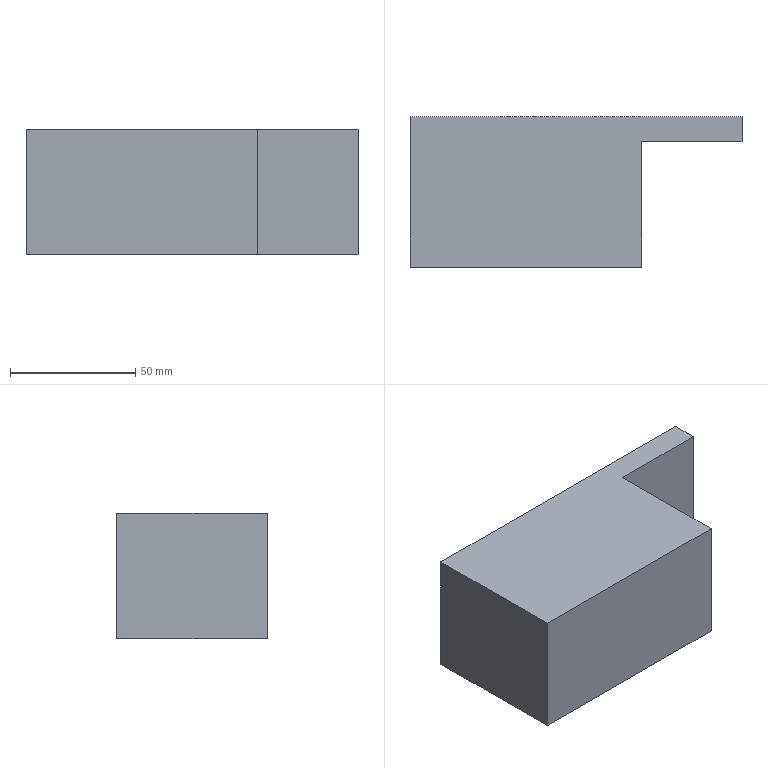Part | NX | features solid 2 | 1 solid | 8 faces | box 132.49 x 60 x 50 mm | volume 297471 mm3 | plane 6 | spline 2
STEP:
#1=CARTESIAN_POINT('',(182.5,350.,70.));
#2=VERTEX_POINT('',#1);
#3=CARTESIAN_POINT('',(90.01,350.,70.));
#4=VERTEX_POINT('',#3);
#5=CARTESIAN_POINT('',(90.01,350.,70.));
#6=CARTESIAN_POINT('',(120.84,350.,70.));
#7=CARTESIAN_POINT('',(151.67,350.,70.));
#8=CARTESIAN_POINT('',(182.5,350.,70.));
#9=B_SPLINE_CURVE_WITH_KNOTS('',3,(#5,#6,#7,#8),.UNSPECIFIED.,.F.,.F.,(4,4),(2.61,2.702),.UNSPECIFIED.);
#10=EDGE_CURVE('',#2,#4,#9,.F.);
#11=ORIENTED_EDGE('',*,*,#10,.T.);
#12=CARTESIAN_POINT('',(90.01,350.,20.));
#13=VERTEX_POINT('',#12);
#14=CARTESIAN_POINT('',(90.01,350.,20.));
#15=CARTESIAN_POINT('',(90.01,350.,36.667));
#16=CARTESIAN_POINT('',(90.01,350.,53.333));
#17=CARTESIAN_POINT('',(90.01,350.,70.));
#18=B_SPLINE_CURVE_WITH_KNOTS('',3,(#14,#15,#16,#17),.UNSPECIFIED.,.F.,.F.,(4,4),(0.,1.),.UNSPECIFIED.);
#19=EDGE_CURVE('',#13,#4,#18,.T.);
#20=ORIENTED_EDGE('',*,*,#19,.F.);
#21=CARTESIAN_POINT('',(182.5,350.,20.));
#22=VERTEX_POINT('',#21);
#23=CARTESIAN_POINT('',(90.01,350.,20.));
#24=CARTESIAN_POINT('',(120.84,350.,20.));
#25=CARTESIAN_POINT('',(151.67,350.,20.));
#26=CARTESIAN_POINT('',(182.5,350.,20.));
#27=B_SPLINE_CURVE_WITH_KNOTS('',3,(#23,#24,#25,#26),.UNSPECIFIED.,.F.,.F.,(4,4),(2.61,2.702),.UNSPECIFIED.);
#28=EDGE_CURVE('',#22,#13,#27,.F.);
#29=ORIENTED_EDGE('',*,*,#28,.F.);
#30=CARTESIAN_POINT('',(182.5,350.,20.));
#31=DIRECTION('',(0.,0.,1.));
#32=VECTOR('',#31,1000.);
#33=LINE('',#30,#32);
#34=EDGE_CURVE('',#22,#2,#33,.T.);
#35=ORIENTED_EDGE('',*,*,#34,.T.);
#36=EDGE_LOOP('',(#11,#20,#29,#35));
#37=FACE_BOUND('',#36,.T.);
#38=CARTESIAN_POINT('',(-270.,350.,20.));
#39=DIRECTION('',(0.,1.,0.));
#40=DIRECTION('',(0.,0.,1.));
#41=AXIS2_PLACEMENT_3D('',#38,#39,#40);
#42=PLANE('',#41);
#43=ADVANCED_FACE('',(#37),#42,.F.);
#44=CARTESIAN_POINT('',(182.5,400.,70.));
#45=VERTEX_POINT('',#44);
#46=CARTESIAN_POINT('',(182.5,490.534,70.));
#47=DIRECTION('',(0.,1.,0.));
#48=VECTOR('',#47,1000.);
#49=LINE('',#46,#48);
#50=EDGE_CURVE('',#2,#45,#49,.T.);
#51=ORIENTED_EDGE('',*,*,#50,.F.);
#52=ORIENTED_EDGE('',*,*,#34,.F.);
#53=CARTESIAN_POINT('',(182.5,400.,20.));
#54=VERTEX_POINT('',#53);
#55=CARTESIAN_POINT('',(182.5,490.534,20.));
#56=DIRECTION('',(0.,1.,0.));
#57=VECTOR('',#56,1000.);
#58=LINE('',#55,#57);
#59=EDGE_CURVE('',#22,#54,#58,.T.);
#60=ORIENTED_EDGE('',*,*,#59,.T.);
#61=CARTESIAN_POINT('',(182.5,400.,20.));
#62=DIRECTION('',(0.,0.,1.));
#63=VECTOR('',#62,1000.);
#64=LINE('',#61,#63);
#65=EDGE_CURVE('',#54,#45,#64,.T.);
#66=ORIENTED_EDGE('',*,*,#65,.T.);
#67=EDGE_LOOP('',(#51,#52,#60,#66));
#68=FACE_BOUND('',#67,.T.);
#69=CARTESIAN_POINT('',(182.5,490.534,20.));
#70=DIRECTION('',(1.,0.,0.));
#71=DIRECTION('',(0.,0.,-1.));
#72=AXIS2_PLACEMENT_3D('',#69,#70,#71);
#73=PLANE('',#72);
#74=ADVANCED_FACE('',(#68),#73,.T.);
#75=CARTESIAN_POINT('',(222.5,400.,70.));
#76=VERTEX_POINT('',#75);
#77=CARTESIAN_POINT('',(182.5,400.,70.));
#78=CARTESIAN_POINT('',(195.833,400.,70.));
#79=CARTESIAN_POINT('',(209.167,400.,70.));
#80=CARTESIAN_POINT('',(222.5,400.,70.));
#81=B_SPLINE_CURVE_WITH_KNOTS('',3,(#77,#78,#79,#80),.UNSPECIFIED.,.F.,.F.,(4,4),(0.,0.04),.UNSPECIFIED.);
#82=EDGE_CURVE('',#45,#76,#81,.T.);
#83=ORIENTED_EDGE('',*,*,#82,.F.);
#84=ORIENTED_EDGE('',*,*,#65,.F.);
#85=CARTESIAN_POINT('',(222.5,400.,20.));
#86=VERTEX_POINT('',#85);
#87=CARTESIAN_POINT('',(182.5,400.,20.));
#88=CARTESIAN_POINT('',(195.833,400.,20.));
#89=CARTESIAN_POINT('',(209.167,400.,20.));
#90=CARTESIAN_POINT('',(222.5,400.,20.));
#91=B_SPLINE_CURVE_WITH_KNOTS('',3,(#87,#88,#89,#90),.UNSPECIFIED.,.F.,.F.,(4,4),(0.,0.04),.UNSPECIFIED.);
#92=EDGE_CURVE('',#54,#86,#91,.T.);
#93=ORIENTED_EDGE('',*,*,#92,.T.);
#94=CARTESIAN_POINT('',(222.5,400.,20.));
#95=DIRECTION('',(0.,0.,1.));
#96=VECTOR('',#95,1000.);
#97=LINE('',#94,#96);
#98=EDGE_CURVE('',#86,#76,#97,.T.);
#99=ORIENTED_EDGE('',*,*,#98,.T.);
#100=EDGE_LOOP('',(#83,#84,#93,#99));
#101=FACE_BOUND('',#100,.T.);
#102=CARTESIAN_POINT('',(182.5,400.,20.));
#103=DIRECTION('',(0.,-1.,0.));
#104=DIRECTION('',(0.,0.,-1.));
#105=AXIS2_PLACEMENT_3D('',#102,#103,#104);
#106=PLANE('',#105);
#107=ADVANCED_FACE('',(#101),#106,.T.);
#108=CARTESIAN_POINT('',(222.5,410.,70.));
#109=VERTEX_POINT('',#108);
#110=CARTESIAN_POINT('',(222.5,400.,70.));
#111=CARTESIAN_POINT('',(222.5,403.333,70.));
#112=CARTESIAN_POINT('',(222.5,406.667,70.));
#113=CARTESIAN_POINT('',(222.5,410.,70.));
#114=B_SPLINE_CURVE_WITH_KNOTS('',3,(#110,#111,#112,#113),.UNSPECIFIED.,.F.,.F.,(4,4),(0.09182,0.1018),.UNSPECIFIED.);
#115=EDGE_CURVE('',#76,#109,#114,.T.);
#116=ORIENTED_EDGE('',*,*,#115,.F.);
#117=ORIENTED_EDGE('',*,*,#98,.F.);
#118=CARTESIAN_POINT('',(222.5,410.,20.));
#119=VERTEX_POINT('',#118);
#120=CARTESIAN_POINT('',(222.5,400.,20.));
#121=CARTESIAN_POINT('',(222.5,403.333,20.));
#122=CARTESIAN_POINT('',(222.5,406.667,20.));
#123=CARTESIAN_POINT('',(222.5,410.,20.));
#124=B_SPLINE_CURVE_WITH_KNOTS('',3,(#120,#121,#122,#123),.UNSPECIFIED.,.F.,.F.,(4,4),(0.09182,0.1018),.UNSPECIFIED.);
#125=EDGE_CURVE('',#86,#119,#124,.T.);
#126=ORIENTED_EDGE('',*,*,#125,.T.);
#127=CARTESIAN_POINT('',(222.5,410.,20.));
#128=DIRECTION('',(0.,0.,1.));
#129=VECTOR('',#128,1000.);
#130=LINE('',#127,#129);
#131=EDGE_CURVE('',#119,#109,#130,.T.);
#132=ORIENTED_EDGE('',*,*,#131,.T.);
#133=EDGE_LOOP('',(#116,#117,#126,#132));
#134=FACE_BOUND('',#133,.T.);
#135=CARTESIAN_POINT('',(222.5,400.,20.));
#136=DIRECTION('',(1.,0.,0.));
#137=DIRECTION('',(0.,0.,-1.));
#138=AXIS2_PLACEMENT_3D('',#135,#136,#137);
#139=PLANE('',#138);
#140=ADVANCED_FACE('',(#134),#139,.T.);
#141=CARTESIAN_POINT('',(90.01,410.,70.));
#142=VERTEX_POINT('',#141);
#143=CARTESIAN_POINT('',(222.5,410.,70.));
#144=CARTESIAN_POINT('',(178.337,410.,70.));
#145=CARTESIAN_POINT('',(134.173,410.,70.));
#146=CARTESIAN_POINT('',(90.01,410.,70.));
#147=B_SPLINE_CURVE_WITH_KNOTS('',3,(#143,#144,#145,#146),.UNSPECIFIED.,.F.,.F.,(4,4),(-0.04,0.09249),.UNSPECIFIED.);
#148=EDGE_CURVE('',#109,#142,#147,.T.);
#149=ORIENTED_EDGE('',*,*,#148,.F.);
#150=ORIENTED_EDGE('',*,*,#131,.F.);
#151=CARTESIAN_POINT('',(90.01,410.,20.));
#152=VERTEX_POINT('',#151);
#153=CARTESIAN_POINT('',(222.5,410.,20.));
#154=CARTESIAN_POINT('',(178.337,410.,20.));
#155=CARTESIAN_POINT('',(134.173,410.,20.));
#156=CARTESIAN_POINT('',(90.01,410.,20.));
#157=B_SPLINE_CURVE_WITH_KNOTS('',3,(#153,#154,#155,#156),.UNSPECIFIED.,.F.,.F.,(4,4),(-0.04,0.09249),.UNSPECIFIED.);
#158=EDGE_CURVE('',#119,#152,#157,.T.);
#159=ORIENTED_EDGE('',*,*,#158,.T.);
#160=CARTESIAN_POINT('',(90.01,410.,70.));
#161=CARTESIAN_POINT('',(90.01,410.,53.333));
#162=CARTESIAN_POINT('',(90.01,410.,36.667));
#163=CARTESIAN_POINT('',(90.01,410.,20.));
#164=B_SPLINE_CURVE_WITH_KNOTS('',3,(#160,#161,#162,#163),.UNSPECIFIED.,.F.,.F.,(4,4),(0.,1.),.UNSPECIFIED.);
#165=EDGE_CURVE('',#152,#142,#164,.F.);
#166=ORIENTED_EDGE('',*,*,#165,.T.);
#167=EDGE_LOOP('',(#149,#150,#159,#166));
#168=FACE_BOUND('',#167,.T.);
#169=CARTESIAN_POINT('',(386.136,410.,20.));
#170=DIRECTION('',(0.,1.,0.));
#171=DIRECTION('',(-1.,0.,0.));
#172=AXIS2_PLACEMENT_3D('',#169,#170,#171);
#173=PLANE('',#172);
#174=ADVANCED_FACE('',(#168),#173,.T.);
#175=CARTESIAN_POINT('',(90.01,410.,70.));
#176=CARTESIAN_POINT('',(90.01,390.,70.));
#177=CARTESIAN_POINT('',(90.01,370.,70.));
#178=CARTESIAN_POINT('',(90.01,350.,70.));
#179=B_SPLINE_CURVE_WITH_KNOTS('',3,(#175,#176,#177,#178),.UNSPECIFIED.,.F.,.F.,(4,4),(0.,1.),.UNSPECIFIED.);
#180=EDGE_CURVE('',#142,#4,#179,.T.);
#181=ORIENTED_EDGE('',*,*,#180,.F.);
#182=ORIENTED_EDGE('',*,*,#165,.F.);
#183=CARTESIAN_POINT('',(90.01,350.,20.));
#184=CARTESIAN_POINT('',(90.01,370.,20.));
#185=CARTESIAN_POINT('',(90.01,390.,20.));
#186=CARTESIAN_POINT('',(90.01,410.,20.));
#187=B_SPLINE_CURVE_WITH_KNOTS('',3,(#183,#184,#185,#186),.UNSPECIFIED.,.F.,.F.,(4,4),(0.,1.),.UNSPECIFIED.);
#188=EDGE_CURVE('',#152,#13,#187,.F.);
#189=ORIENTED_EDGE('',*,*,#188,.T.);
#190=ORIENTED_EDGE('',*,*,#19,.T.);
#191=EDGE_LOOP('',(#181,#182,#189,#190));
#192=FACE_BOUND('',#191,.T.);
#193=CARTESIAN_POINT('',(90.01,490.534,20.));
#194=DIRECTION('',(-1.,0.,0.));
#195=DIRECTION('',(0.,0.,1.));
#196=AXIS2_PLACEMENT_3D('',#193,#194,#195);
#197=PLANE('',#196);
#198=ADVANCED_FACE('',(#192),#197,.T.);
#199=ORIENTED_EDGE('',*,*,#28,.T.);
#200=ORIENTED_EDGE('',*,*,#188,.F.);
#201=ORIENTED_EDGE('',*,*,#158,.F.);
#202=ORIENTED_EDGE('',*,*,#125,.F.);
#203=ORIENTED_EDGE('',*,*,#92,.F.);
#204=ORIENTED_EDGE('',*,*,#59,.F.);
#205=EDGE_LOOP('',(#199,#200,#201,#202,#203,#204));
#206=FACE_BOUND('',#205,.T.);
#207=CARTESIAN_POINT('',(222.5,349.64,20.));
#208=CARTESIAN_POINT('',(90.01,349.64,20.));
#209=CARTESIAN_POINT('',(222.5,410.,20.));
#210=CARTESIAN_POINT('',(90.01,410.,20.));
#211=B_SPLINE_SURFACE_WITH_KNOTS('',1,1,((#207,#208),(#209,#210)),.PLANE_SURF.,.F.,.F.,.F.,(2,2),(2,2),(0.1032,0.2603),(0.1027,0.3393),.PIECEWISE_BEZIER_KNOTS.);
#212=ADVANCED_FACE('',(#206),#211,.F.);
#213=ORIENTED_EDGE('',*,*,#10,.F.);
#214=ORIENTED_EDGE('',*,*,#50,.T.);
#215=ORIENTED_EDGE('',*,*,#82,.T.);
#216=ORIENTED_EDGE('',*,*,#115,.T.);
#217=ORIENTED_EDGE('',*,*,#148,.T.);
#218=ORIENTED_EDGE('',*,*,#180,.T.);
#219=EDGE_LOOP('',(#213,#214,#215,#216,#217,#218));
#220=FACE_BOUND('',#219,.T.);
#221=CARTESIAN_POINT('',(222.5,349.64,70.));
#222=CARTESIAN_POINT('',(90.01,349.64,70.));
#223=CARTESIAN_POINT('',(222.5,410.,70.));
#224=CARTESIAN_POINT('',(90.01,410.,70.));
#225=B_SPLINE_SURFACE_WITH_KNOTS('',1,1,((#221,#222),(#223,#224)),.PLANE_SURF.,.F.,.F.,.F.,(2,2),(2,2),(0.1032,0.2603),(0.1027,0.3393),.PIECEWISE_BEZIER_KNOTS.);
#226=ADVANCED_FACE('',(#220),#225,.T.);
#227=CLOSED_SHELL('',(#43,#74,#107,#140,#174,#198,#212,#226));
#228=MANIFOLD_SOLID_BREP('',#227);
#229=(LENGTH_UNIT()NAMED_UNIT(*)SI_UNIT(.MILLI.,.METRE.));
#230=UNCERTAINTY_MEASURE_WITH_UNIT(LENGTH_MEASURE(0.0508),#229,'','');
#231=(NAMED_UNIT(*)PLANE_ANGLE_UNIT()SI_UNIT($,.RADIAN.));
#232=(NAMED_UNIT(*)SI_UNIT($,.STERADIAN.)SOLID_ANGLE_UNIT());
#233=(GEOMETRIC_REPRESENTATION_CONTEXT(3)GLOBAL_UNCERTAINTY_ASSIGNED_CONTEXT((#230))GLOBAL_UNIT_ASSIGNED_CONTEXT((#229,#231,#232))REPRESENTATION_CONTEXT('',''));
#234=ADVANCED_BREP_SHAPE_REPRESENTATION('',(#228),#233);